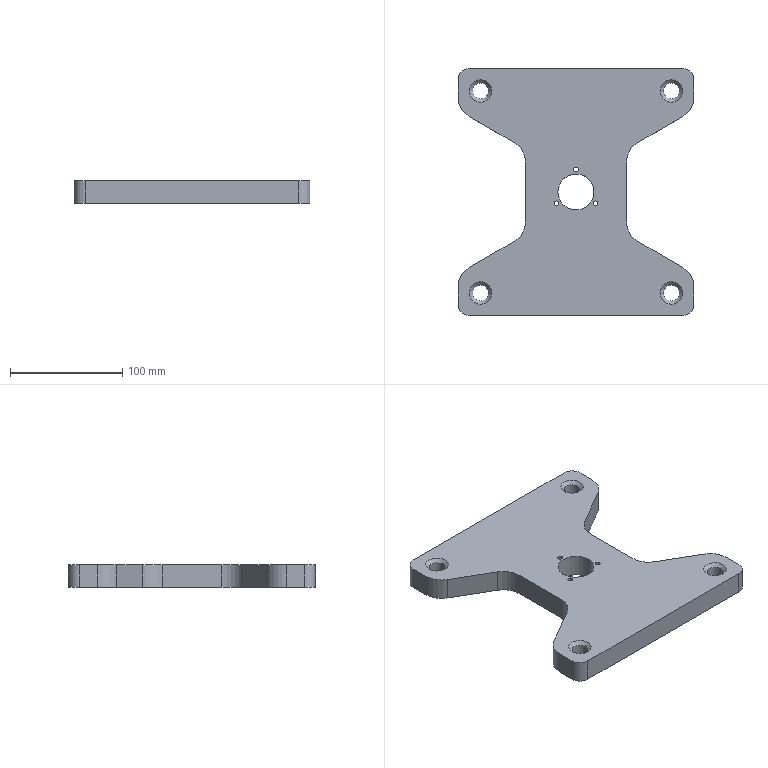Part | STEP file | YBQDJ-YL-6 | 1 solid | 56 faces | box 210 x 220 x 20 mm | volume 625567 mm3 | cylinder 35 | plane 14 | cone 7 | commonest cylinder face diameters 4 x10 40 x8 1 x5 14 x4 20 x4 4.2 x3